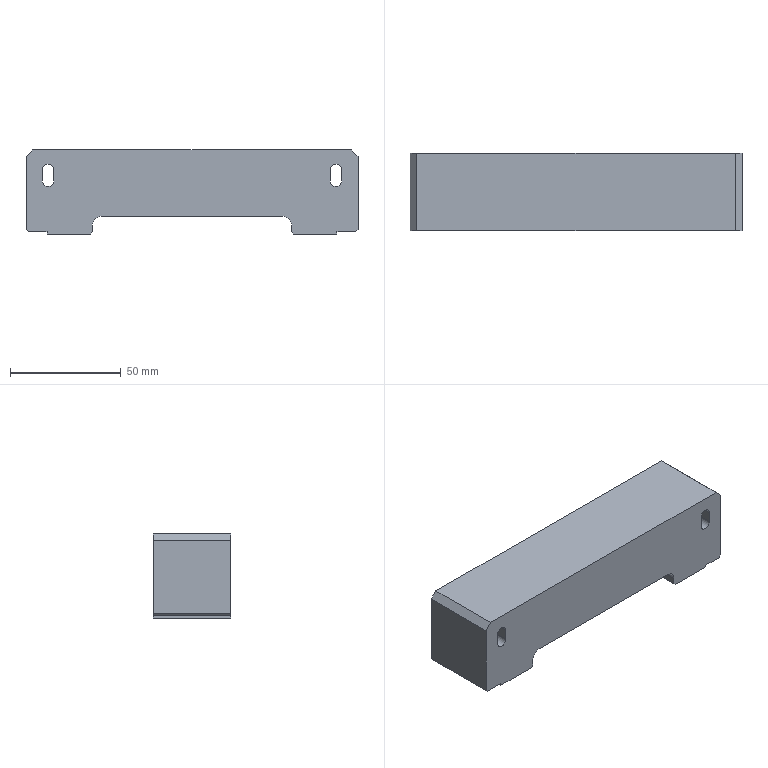Part | STEP file | linear rail mounting plate | 1 solid | 68 faces | box 150 x 35 x 38 mm | volume 166586 mm3 | plane 30 | cylinder 26 | cone 12 | commonest cylinder face diameters 2.5 x12 5.2 x6 10 x6 8 x2